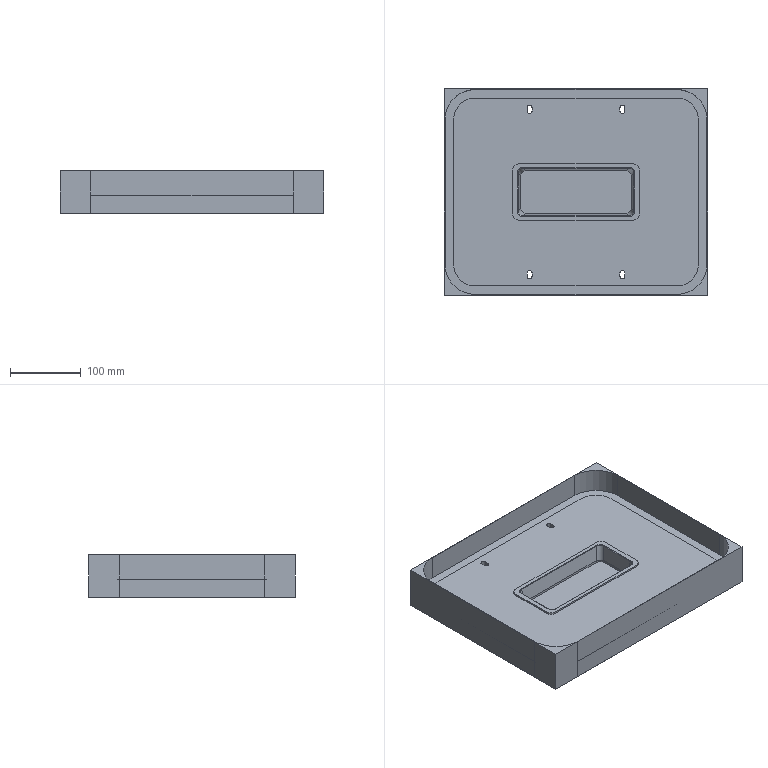Part | 4 solids | 101 faces | box 371 x 291 x 60.5 mm | volume 2672131 mm3 | plane 53 | cylinder 36 | spline 12 | commonest cylinder face diameters 7 x8 60 x8 84 x8 1.9 x4 14.1 x4 18 x4